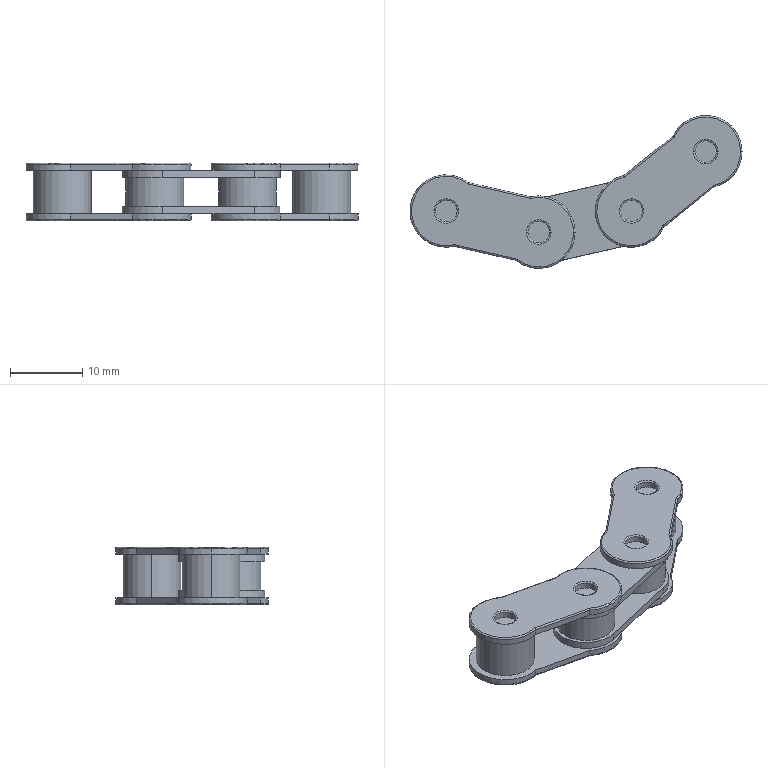Part | STEP file | Idler Chain v2 | 1 solid | 110 faces | box 45.864 x 21.107 x 8 mm | volume 2108 mm3 | cylinder 50 | plane 32 | torus 28 | commonest cylinder face diameters 3 x16 10 x12 0.4 x8 8 x8 9 x6